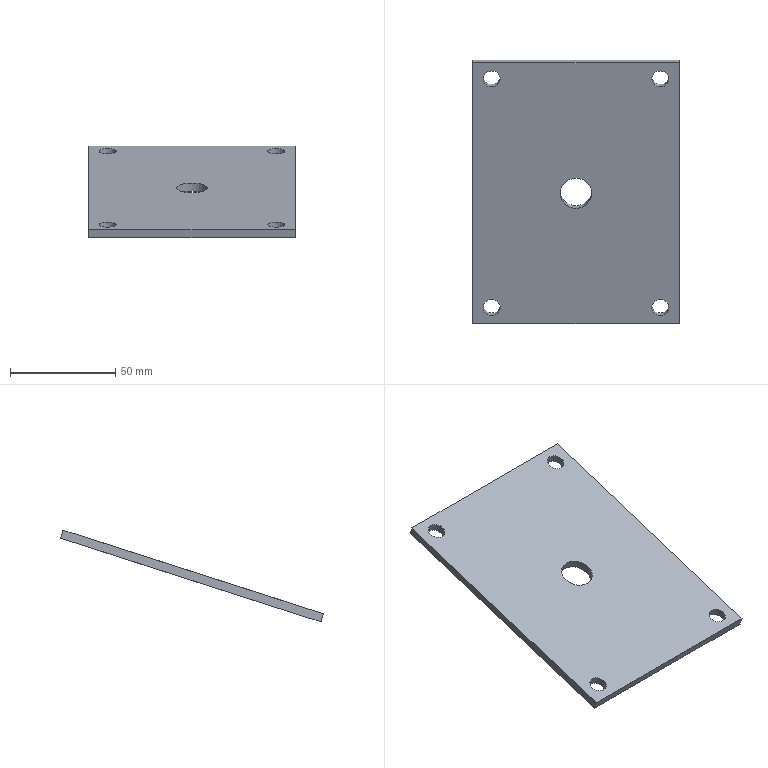Part | NX | features DATUM_CSYS 43, EXTRUDE 42, SKETCH 42, EXTRACT_DATUM_AXIS 38, EXTRACT_FACE 32, SIMPLE HOLE 20, EXTRACT_DATUM_PLANE 14, Instance Feature 13, DRAFT 9, EXTRACT_STRING 8, HOLE PACKAGE 7, FSET 6, Mirror Feature 5, BLEND 4, OFFSET_REGION 4, Pattern Feature 2, REPLACE_FACE 1, TRIM BODY 1 | 1 solid | 11 faces | box 98 x 124.993 x 43.573 mm | volume 49449 mm3 | plane 6 | cylinder 5 | commonest cylinder face diameters 8 x4 15 x1
STEP:
#1=CARTESIAN_POINT('',(0.,52.376,126.063));
#2=VERTEX_POINT('',#1);
#3=CARTESIAN_POINT('',(0.,45.235,123.769));
#4=DIRECTION('',(0.,0.3059,-0.9521));
#5=DIRECTION('',(0.,0.9521,0.3059));
#6=AXIS2_PLACEMENT_3D('',#3,#4,#5);
#7=CIRCLE('',#6,7.5);
#8=EDGE_CURVE('',#2,#2,#7,.T.);
#9=ORIENTED_EDGE('',*,*,#8,.F.);
#10=EDGE_LOOP('',(#9));
#11=FACE_BOUND('',#10,.T.);
#12=CARTESIAN_POINT('',(-49.,107.12,143.651));
#13=VERTEX_POINT('',#12);
#14=CARTESIAN_POINT('',(-49.,-16.649,103.887));
#15=VERTEX_POINT('',#14);
#16=CARTESIAN_POINT('',(-49.,107.12,143.651));
#17=DIRECTION('',(0.,-0.9521,-0.3059));
#18=VECTOR('',#17,1000.);
#19=LINE('',#16,#18);
#20=EDGE_CURVE('',#13,#15,#19,.T.);
#21=ORIENTED_EDGE('',*,*,#20,.F.);
#22=CARTESIAN_POINT('',(49.,107.12,143.651));
#23=VERTEX_POINT('',#22);
#24=CARTESIAN_POINT('',(49.,107.12,143.651));
#25=DIRECTION('',(-1.,0.,0.));
#26=VECTOR('',#25,1000.);
#27=LINE('',#24,#26);
#28=EDGE_CURVE('',#23,#13,#27,.T.);
#29=ORIENTED_EDGE('',*,*,#28,.F.);
#30=CARTESIAN_POINT('',(49.,-16.649,103.887));
#31=VERTEX_POINT('',#30);
#32=CARTESIAN_POINT('',(49.,-16.649,103.887));
#33=DIRECTION('',(0.,0.9521,0.3059));
#34=VECTOR('',#33,1000.);
#35=LINE('',#32,#34);
#36=EDGE_CURVE('',#31,#23,#35,.T.);
#37=ORIENTED_EDGE('',*,*,#36,.F.);
#38=CARTESIAN_POINT('',(-49.,-16.649,103.887));
#39=DIRECTION('',(1.,0.,0.));
#40=VECTOR('',#39,1000.);
#41=LINE('',#38,#40);
#42=EDGE_CURVE('',#15,#31,#41,.T.);
#43=ORIENTED_EDGE('',*,*,#42,.F.);
#44=EDGE_LOOP('',(#21,#29,#37,#43));
#45=FACE_BOUND('',#44,.T.);
#46=CARTESIAN_POINT('',(-40.,-5.224,107.557));
#47=VERTEX_POINT('',#46);
#48=CARTESIAN_POINT('',(-40.,-9.033,106.334));
#49=DIRECTION('',(0.,0.3059,-0.9521));
#50=DIRECTION('',(0.,0.9521,0.3059));
#51=AXIS2_PLACEMENT_3D('',#48,#49,#50);
#52=CIRCLE('',#51,4.);
#53=EDGE_CURVE('',#47,#47,#52,.F.);
#54=ORIENTED_EDGE('',*,*,#53,.T.);
#55=EDGE_LOOP('',(#54));
#56=FACE_BOUND('',#55,.T.);
#57=CARTESIAN_POINT('',(40.,-5.224,107.557));
#58=VERTEX_POINT('',#57);
#59=CARTESIAN_POINT('',(40.,-9.033,106.334));
#60=DIRECTION('',(0.,0.3059,-0.9521));
#61=DIRECTION('',(0.,0.9521,0.3059));
#62=AXIS2_PLACEMENT_3D('',#59,#60,#61);
#63=CIRCLE('',#62,4.);
#64=EDGE_CURVE('',#58,#58,#63,.T.);
#65=ORIENTED_EDGE('',*,*,#64,.F.);
#66=EDGE_LOOP('',(#65));
#67=FACE_BOUND('',#66,.T.);
#68=CARTESIAN_POINT('',(-40.,103.312,142.428));
#69=VERTEX_POINT('',#68);
#70=CARTESIAN_POINT('',(-40.,99.503,141.204));
#71=DIRECTION('',(0.,0.3059,-0.9521));
#72=DIRECTION('',(0.,0.9521,0.3059));
#73=AXIS2_PLACEMENT_3D('',#70,#71,#72);
#74=CIRCLE('',#73,4.);
#75=EDGE_CURVE('',#69,#69,#74,.T.);
#76=ORIENTED_EDGE('',*,*,#75,.F.);
#77=EDGE_LOOP('',(#76));
#78=FACE_BOUND('',#77,.T.);
#79=CARTESIAN_POINT('',(40.,103.312,142.428));
#80=VERTEX_POINT('',#79);
#81=CARTESIAN_POINT('',(40.,99.503,141.204));
#82=DIRECTION('',(0.,0.3059,-0.9521));
#83=DIRECTION('',(0.,0.9521,0.3059));
#84=AXIS2_PLACEMENT_3D('',#81,#82,#83);
#85=CIRCLE('',#84,4.);
#86=EDGE_CURVE('',#80,#80,#85,.F.);
#87=ORIENTED_EDGE('',*,*,#86,.T.);
#88=EDGE_LOOP('',(#87));
#89=FACE_BOUND('',#88,.T.);
#90=CARTESIAN_POINT('',(0.,45.235,123.769));
#91=DIRECTION('',(0.,0.3059,-0.9521));
#92=DIRECTION('',(0.,0.9521,0.3059));
#93=AXIS2_PLACEMENT_3D('',#90,#91,#92);
#94=PLANE('',#93);
#95=ADVANCED_FACE('',(#11,#45,#56,#67,#78,#89),#94,.T.);
#96=CARTESIAN_POINT('',(40.,102.088,146.236));
#97=VERTEX_POINT('',#96);
#98=CARTESIAN_POINT('',(40.,98.28,145.013));
#99=DIRECTION('',(0.,0.3059,-0.9521));
#100=DIRECTION('',(0.,0.9521,0.3059));
#101=AXIS2_PLACEMENT_3D('',#98,#99,#100);
#102=CIRCLE('',#101,4.);
#103=EDGE_CURVE('',#97,#97,#102,.T.);
#104=ORIENTED_EDGE('',*,*,#103,.F.);
#105=EDGE_LOOP('',(#104));
#106=FACE_BOUND('',#105,.T.);
#107=ORIENTED_EDGE('',*,*,#86,.F.);
#108=EDGE_LOOP('',(#107));
#109=FACE_BOUND('',#108,.T.);
#110=CARTESIAN_POINT('',(40.,98.28,145.013));
#111=DIRECTION('',(0.,0.3059,-0.9521));
#112=DIRECTION('',(0.,0.9521,0.3059));
#113=AXIS2_PLACEMENT_3D('',#110,#111,#112);
#114=CYLINDRICAL_SURFACE('',#113,4.);
#115=ADVANCED_FACE('',(#106,#109),#114,.F.);
#116=CARTESIAN_POINT('',(-40.,102.088,146.236));
#117=VERTEX_POINT('',#116);
#118=CARTESIAN_POINT('',(-40.,98.28,145.013));
#119=DIRECTION('',(0.,-0.3059,0.9521));
#120=DIRECTION('',(0.,0.9521,0.3059));
#121=AXIS2_PLACEMENT_3D('',#118,#119,#120);
#122=CIRCLE('',#121,4.);
#123=EDGE_CURVE('',#117,#117,#122,.T.);
#124=ORIENTED_EDGE('',*,*,#123,.T.);
#125=EDGE_LOOP('',(#124));
#126=FACE_BOUND('',#125,.T.);
#127=ORIENTED_EDGE('',*,*,#75,.T.);
#128=EDGE_LOOP('',(#127));
#129=FACE_BOUND('',#128,.T.);
#130=CARTESIAN_POINT('',(-40.,98.28,145.013));
#131=DIRECTION('',(0.,0.3059,-0.9521));
#132=DIRECTION('',(0.,0.9521,0.3059));
#133=AXIS2_PLACEMENT_3D('',#130,#131,#132);
#134=CYLINDRICAL_SURFACE('',#133,4.);
#135=ADVANCED_FACE('',(#126,#129),#134,.F.);
#136=CARTESIAN_POINT('',(-40.,-14.064,108.918));
#137=VERTEX_POINT('',#136);
#138=CARTESIAN_POINT('',(-40.,-10.256,110.142));
#139=DIRECTION('',(0.,0.3059,-0.9521));
#140=DIRECTION('',(0.,-0.9521,-0.3059));
#141=AXIS2_PLACEMENT_3D('',#138,#139,#140);
#142=CIRCLE('',#141,4.);
#143=EDGE_CURVE('',#137,#137,#142,.T.);
#144=ORIENTED_EDGE('',*,*,#143,.F.);
#145=EDGE_LOOP('',(#144));
#146=FACE_BOUND('',#145,.T.);
#147=ORIENTED_EDGE('',*,*,#53,.F.);
#148=EDGE_LOOP('',(#147));
#149=FACE_BOUND('',#148,.T.);
#150=CARTESIAN_POINT('',(-40.,-10.256,110.142));
#151=DIRECTION('',(0.,0.3059,-0.9521));
#152=DIRECTION('',(0.,0.9521,0.3059));
#153=AXIS2_PLACEMENT_3D('',#150,#151,#152);
#154=CYLINDRICAL_SURFACE('',#153,4.);
#155=ADVANCED_FACE('',(#146,#149),#154,.F.);
#156=CARTESIAN_POINT('',(40.,-14.064,108.918));
#157=VERTEX_POINT('',#156);
#158=CARTESIAN_POINT('',(40.,-10.256,110.142));
#159=DIRECTION('',(0.,-0.3059,0.9521));
#160=DIRECTION('',(0.,-0.9521,-0.3059));
#161=AXIS2_PLACEMENT_3D('',#158,#159,#160);
#162=CIRCLE('',#161,4.);
#163=EDGE_CURVE('',#157,#157,#162,.T.);
#164=ORIENTED_EDGE('',*,*,#163,.T.);
#165=EDGE_LOOP('',(#164));
#166=FACE_BOUND('',#165,.T.);
#167=ORIENTED_EDGE('',*,*,#64,.T.);
#168=EDGE_LOOP('',(#167));
#169=FACE_BOUND('',#168,.T.);
#170=CARTESIAN_POINT('',(40.,-10.256,110.142));
#171=DIRECTION('',(0.,0.3059,-0.9521));
#172=DIRECTION('',(0.,0.9521,0.3059));
#173=AXIS2_PLACEMENT_3D('',#170,#171,#172);
#174=CYLINDRICAL_SURFACE('',#173,4.);
#175=ADVANCED_FACE('',(#166,#169),#174,.F.);
#176=ORIENTED_EDGE('',*,*,#20,.T.);
#177=CARTESIAN_POINT('',(-49.,-17.873,107.695));
#178=VERTEX_POINT('',#177);
#179=CARTESIAN_POINT('',(-49.,-17.873,107.695));
#180=DIRECTION('',(0.,0.3059,-0.9521));
#181=VECTOR('',#180,1000.);
#182=LINE('',#179,#181);
#183=EDGE_CURVE('',#178,#15,#182,.T.);
#184=ORIENTED_EDGE('',*,*,#183,.F.);
#185=CARTESIAN_POINT('',(-49.,105.896,147.46));
#186=VERTEX_POINT('',#185);
#187=CARTESIAN_POINT('',(-49.,105.896,147.46));
#188=DIRECTION('',(0.,-0.9521,-0.3059));
#189=VECTOR('',#188,1000.);
#190=LINE('',#187,#189);
#191=EDGE_CURVE('',#186,#178,#190,.T.);
#192=ORIENTED_EDGE('',*,*,#191,.F.);
#193=CARTESIAN_POINT('',(-49.,105.896,147.46));
#194=DIRECTION('',(0.,0.3059,-0.9521));
#195=VECTOR('',#194,1000.);
#196=LINE('',#193,#195);
#197=EDGE_CURVE('',#186,#13,#196,.T.);
#198=ORIENTED_EDGE('',*,*,#197,.T.);
#199=EDGE_LOOP('',(#176,#184,#192,#198));
#200=FACE_BOUND('',#199,.T.);
#201=CARTESIAN_POINT('',(-49.,105.896,147.46));
#202=DIRECTION('',(1.,0.,0.));
#203=DIRECTION('',(0.,0.,-1.));
#204=AXIS2_PLACEMENT_3D('',#201,#202,#203);
#205=PLANE('',#204);
#206=ADVANCED_FACE('',(#200),#205,.F.);
#207=ORIENTED_EDGE('',*,*,#42,.T.);
#208=CARTESIAN_POINT('',(49.,-17.873,107.695));
#209=VERTEX_POINT('',#208);
#210=CARTESIAN_POINT('',(49.,-17.873,107.695));
#211=DIRECTION('',(0.,0.3059,-0.9521));
#212=VECTOR('',#211,1000.);
#213=LINE('',#210,#212);
#214=EDGE_CURVE('',#209,#31,#213,.T.);
#215=ORIENTED_EDGE('',*,*,#214,.F.);
#216=CARTESIAN_POINT('',(-49.,-17.873,107.695));
#217=DIRECTION('',(1.,0.,0.));
#218=VECTOR('',#217,1000.);
#219=LINE('',#216,#218);
#220=EDGE_CURVE('',#178,#209,#219,.T.);
#221=ORIENTED_EDGE('',*,*,#220,.F.);
#222=ORIENTED_EDGE('',*,*,#183,.T.);
#223=EDGE_LOOP('',(#207,#215,#221,#222));
#224=FACE_BOUND('',#223,.T.);
#225=CARTESIAN_POINT('',(-49.,-17.873,107.695));
#226=DIRECTION('',(0.,0.9521,0.3059));
#227=DIRECTION('',(0.,-0.3059,0.9521));
#228=AXIS2_PLACEMENT_3D('',#225,#226,#227);
#229=PLANE('',#228);
#230=ADVANCED_FACE('',(#224),#229,.F.);
#231=ORIENTED_EDGE('',*,*,#36,.T.);
#232=CARTESIAN_POINT('',(49.,105.896,147.46));
#233=VERTEX_POINT('',#232);
#234=CARTESIAN_POINT('',(49.,105.896,147.46));
#235=DIRECTION('',(0.,0.3059,-0.9521));
#236=VECTOR('',#235,1000.);
#237=LINE('',#234,#236);
#238=EDGE_CURVE('',#233,#23,#237,.T.);
#239=ORIENTED_EDGE('',*,*,#238,.F.);
#240=CARTESIAN_POINT('',(49.,-17.873,107.695));
#241=DIRECTION('',(0.,0.9521,0.3059));
#242=VECTOR('',#241,1000.);
#243=LINE('',#240,#242);
#244=EDGE_CURVE('',#209,#233,#243,.T.);
#245=ORIENTED_EDGE('',*,*,#244,.F.);
#246=ORIENTED_EDGE('',*,*,#214,.T.);
#247=EDGE_LOOP('',(#231,#239,#245,#246));
#248=FACE_BOUND('',#247,.T.);
#249=CARTESIAN_POINT('',(49.,-17.873,107.695));
#250=DIRECTION('',(-1.,0.,0.));
#251=DIRECTION('',(0.,0.,1.));
#252=AXIS2_PLACEMENT_3D('',#249,#250,#251);
#253=PLANE('',#252);
#254=ADVANCED_FACE('',(#248),#253,.F.);
#255=ORIENTED_EDGE('',*,*,#28,.T.);
#256=ORIENTED_EDGE('',*,*,#197,.F.);
#257=CARTESIAN_POINT('',(49.,105.896,147.46));
#258=DIRECTION('',(-1.,0.,0.));
#259=VECTOR('',#258,1000.);
#260=LINE('',#257,#259);
#261=EDGE_CURVE('',#233,#186,#260,.T.);
#262=ORIENTED_EDGE('',*,*,#261,.F.);
#263=ORIENTED_EDGE('',*,*,#238,.T.);
#264=EDGE_LOOP('',(#255,#256,#262,#263));
#265=FACE_BOUND('',#264,.T.);
#266=CARTESIAN_POINT('',(49.,105.896,147.46));
#267=DIRECTION('',(0.,-0.9521,-0.3059));
#268=DIRECTION('',(0.,0.3059,-0.9521));
#269=AXIS2_PLACEMENT_3D('',#266,#267,#268);
#270=PLANE('',#269);
#271=ADVANCED_FACE('',(#265),#270,.F.);
#272=CARTESIAN_POINT('',(0.,51.152,129.871));
#273=VERTEX_POINT('',#272);
#274=CARTESIAN_POINT('',(0.,44.012,127.577));
#275=DIRECTION('',(0.,-0.3059,0.9521));
#276=DIRECTION('',(0.,0.9521,0.3059));
#277=AXIS2_PLACEMENT_3D('',#274,#275,#276);
#278=CIRCLE('',#277,7.5);
#279=EDGE_CURVE('',#273,#273,#278,.T.);
#280=ORIENTED_EDGE('',*,*,#279,.F.);
#281=EDGE_LOOP('',(#280));
#282=FACE_BOUND('',#281,.T.);
#283=ORIENTED_EDGE('',*,*,#191,.T.);
#284=ORIENTED_EDGE('',*,*,#220,.T.);
#285=ORIENTED_EDGE('',*,*,#244,.T.);
#286=ORIENTED_EDGE('',*,*,#261,.T.);
#287=EDGE_LOOP('',(#283,#284,#285,#286));
#288=FACE_BOUND('',#287,.T.);
#289=ORIENTED_EDGE('',*,*,#103,.T.);
#290=EDGE_LOOP('',(#289));
#291=FACE_BOUND('',#290,.T.);
#292=ORIENTED_EDGE('',*,*,#163,.F.);
#293=EDGE_LOOP('',(#292));
#294=FACE_BOUND('',#293,.T.);
#295=ORIENTED_EDGE('',*,*,#123,.F.);
#296=EDGE_LOOP('',(#295));
#297=FACE_BOUND('',#296,.T.);
#298=ORIENTED_EDGE('',*,*,#143,.T.);
#299=EDGE_LOOP('',(#298));
#300=FACE_BOUND('',#299,.T.);
#301=CARTESIAN_POINT('',(40.,98.28,145.013));
#302=DIRECTION('',(0.,0.3059,-0.9521));
#303=DIRECTION('',(0.,0.9521,0.3059));
#304=AXIS2_PLACEMENT_3D('',#301,#302,#303);
#305=PLANE('',#304);
#306=ADVANCED_FACE('',(#282,#288,#291,#294,#297,#300),#305,.F.);
#307=ORIENTED_EDGE('',*,*,#8,.T.);
#308=EDGE_LOOP('',(#307));
#309=FACE_BOUND('',#308,.T.);
#310=ORIENTED_EDGE('',*,*,#279,.T.);
#311=EDGE_LOOP('',(#310));
#312=FACE_BOUND('',#311,.T.);
#313=CARTESIAN_POINT('',(0.,53.188,99.015));
#314=DIRECTION('',(0.,-0.3059,0.9521));
#315=DIRECTION('',(0.,-0.9521,-0.3059));
#316=AXIS2_PLACEMENT_3D('',#313,#314,#315);
#317=CYLINDRICAL_SURFACE('',#316,7.5);
#318=ADVANCED_FACE('',(#309,#312),#317,.F.);
#319=CLOSED_SHELL('',(#95,#115,#135,#155,#175,#206,#230,#254,#271,#306,#318));
#320=MANIFOLD_SOLID_BREP('',#319);
#321=(LENGTH_UNIT()NAMED_UNIT(*)SI_UNIT(.MILLI.,.METRE.));
#322=UNCERTAINTY_MEASURE_WITH_UNIT(LENGTH_MEASURE(0.00001),#321,'','');
#323=(NAMED_UNIT(*)PLANE_ANGLE_UNIT()SI_UNIT($,.RADIAN.));
#324=(NAMED_UNIT(*)SI_UNIT($,.STERADIAN.)SOLID_ANGLE_UNIT());
#325=(GEOMETRIC_REPRESENTATION_CONTEXT(3)GLOBAL_UNCERTAINTY_ASSIGNED_CONTEXT((#322))GLOBAL_UNIT_ASSIGNED_CONTEXT((#321,#323,#324))REPRESENTATION_CONTEXT('',''));
#326=ADVANCED_BREP_SHAPE_REPRESENTATION('',(#320),#325);